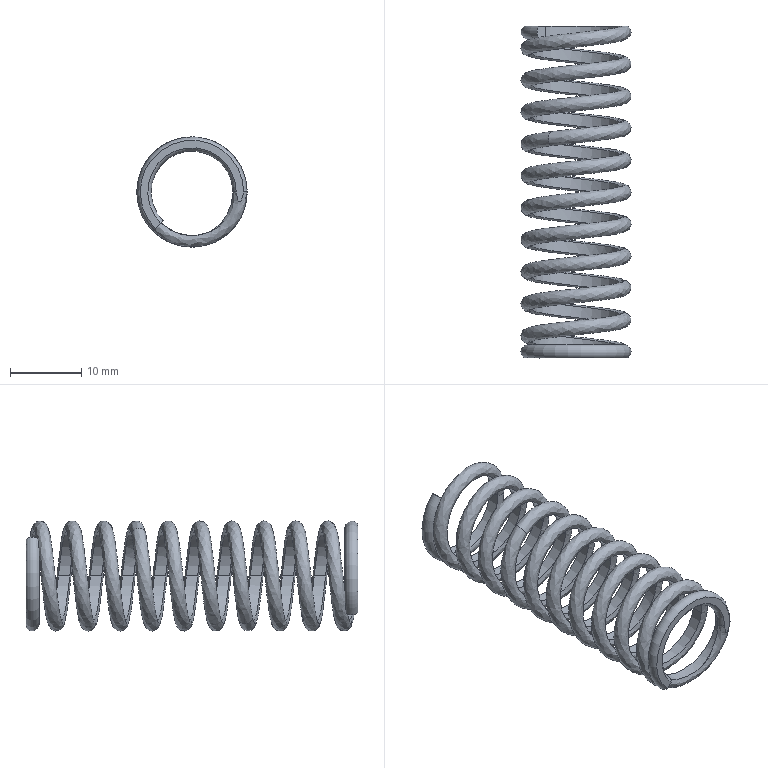Part | Creo | features DATUM PLANE 4, PROTRUSION 3, CURVE 2, CUT 2, COORDINATE SYSTEM 1 | 1 solid | 34 faces | volume 1308 mm3 | cylinder 22 | plane 5 | torus 4 | spline 3 | commonest cylinder face diameters 12.3 x22